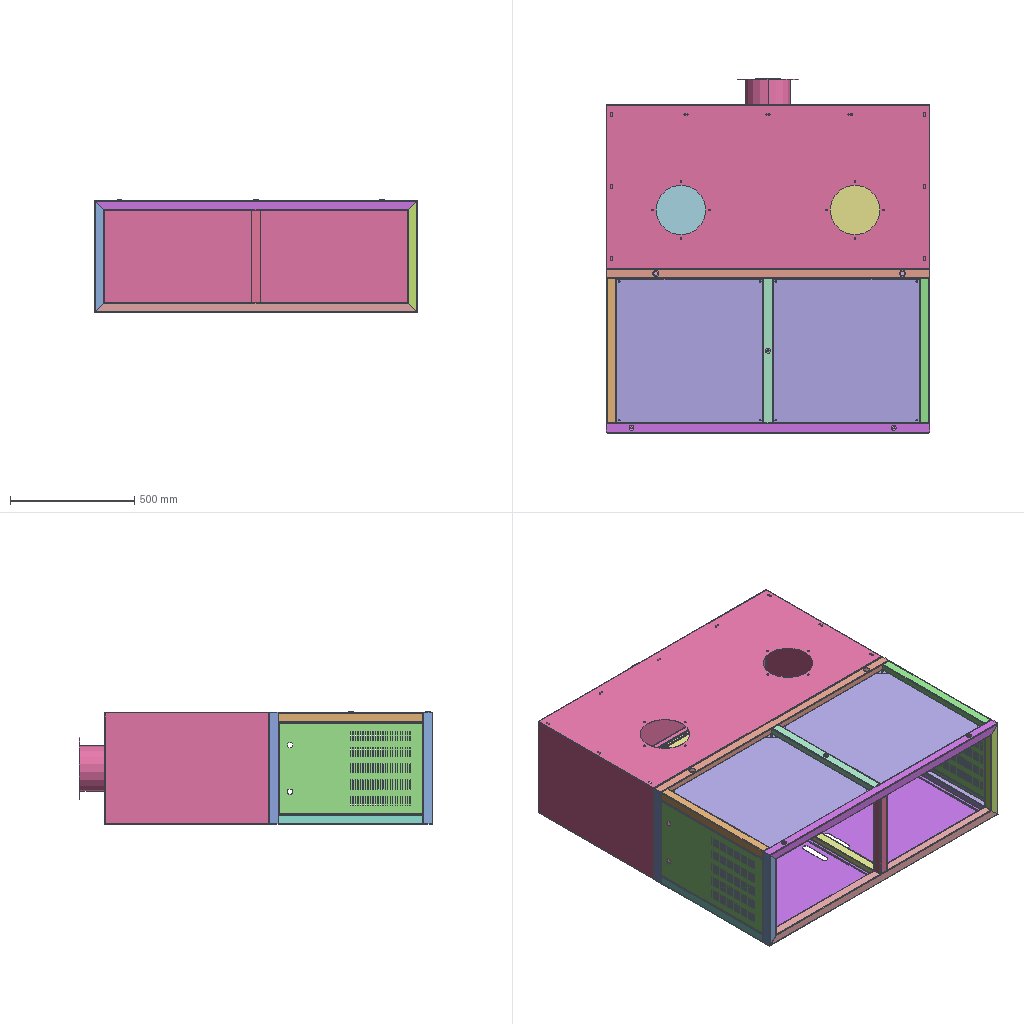Assembly | SolidWorks | 9 different items | 19 placed | box 1300 x 1423 x 453 mm
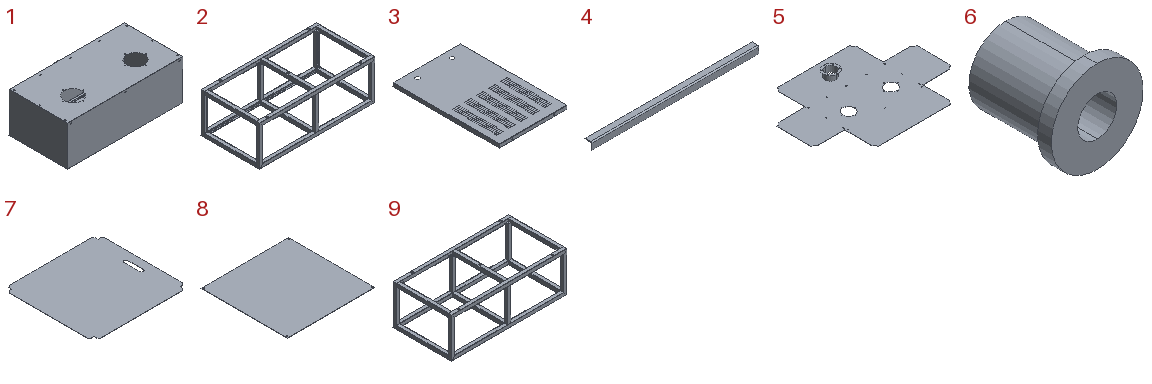Parts list (item | name | quantity | parent item | size | volume | features):
1 | (subassembly) | x1 | - | 1300 x 763 x 450 mm | 5569322 mm3 | -
2 | (subassembly) | x1 | - | 1300 x 660 x 453 mm | 3352763 mm3 | -
3 | - | x2 | - | 367 x 577 x 20 mm | 391645 mm3 | features Cut 3, EdgeFlange 2, LPattern 2, FlatPattern 1, ICE 1, SMBaseFlange 1, SheetMetal 1
4 | - | x4 | in 2 | 360 x 15 x 15 mm | 15045 mm3 | features EdgeFlange 1, FlatPattern 1, SMBaseFlange 1, SheetMetal 1
5 | - | x1 | in 1 | 2323 x 1683 x 104.5 mm | 4309239 mm3 | features ICE 8, EdgeFlange 4, CirPattern 1, FlatPattern 1, SMBaseFlange 1, SheetMetal 1
6 | - | x3 | in 2 | 20 x 20 x 20 mm | 3226 mm3 | features Extrusion 1, HoleWzd 1, ICE 1
7 | - | x4 | in 1 | 668.448 x 638.448 x 1.5 mm | 627538 mm3 | features EdgeFlange 2, FlatPattern 1, ICE 1, SMBaseFlange 1, SheetMetal 1
8 | - | x2 | - | 587 x 577 x 2 mm | 677090 mm3 | features FlatPattern 1, HoleWzd 1, SMBaseFlange 1, SheetMetal 1
9 | - | x1 | in 2 | 1300 x 660 x 450 mm | 3264516 mm3 | features WeldCornerFeat 9, Gusset 8, ICE 3, WeldMemberFeat 3, 3DProfileFeature 1, HoleWzd 1, WeldmentFeature 1
Mates (type | each side: item.copy, entity, surface, feature):
In the top assembly
Width | 8.1 face plane Base-Flange1 | 8.1 face plane Base-Flange1 | 9.1 face plane Structural Member3 | 9.1 face plane Structural Member3
Width | 8.1 face plane Base-Flange1 | 8.1 face plane Base-Flange1 | 9.1 face plane Structural Member1 | 9.1 face plane Structural Member2
Coincident | 9.1 face plane Gusset3 | 8.1 face plane Base-Flange1
Width | 8.2 face plane Base-Flange1 | 8.2 face plane Base-Flange1 | 9.1 face plane Structural Member3 | 9.1 face plane Structural Member3
Width | 8.2 face plane Base-Flange1 | 8.2 face plane Base-Flange1 | 9.1 face plane Structural Member1 | 9.1 face plane Structural Member2
Coincident | 9.1 face plane Gusset6 | 8.2 face plane Base-Flange1
Width | 3.1 face plane Edge-Flange1 | 3.1 face plane Edge-Flange1 | 9.1 face plane Structural Member3 | 9.1 face plane Structural Member3
Width | 3.1 face plane Edge-Flange1 | 3.1 face plane Edge-Flange1 | 9.1 face plane Structural Member1 | 9.1 face plane Structural Member2
Coincident | 9.1 face plane Structural Member2 | 3.1 face plane Base-Flange1
Width | 3.2 face plane Edge-Flange1 | 3.2 face plane Edge-Flange1 | 9.1 face plane Structural Member3 | 9.1 face plane Structural Member3
Coincident | 9.1 face plane Structural Member2 | 3.2 face plane Base-Flange1
Width | 3.2 face plane Edge-Flange1 | 3.2 face plane Edge-Flange1 | 9.1 face plane Structural Member1 | 9.1 face plane Structural Member2
Coincident | 9.1 face plane Structural Member2 | 5.1 face plane Edge-Flange1 | 2 times
Coincident | 9.1 face plane Structural Member2 | 5.1 face plane Edge-Flange2
Width | 7.1 face plane Edge-Flange1 | 7.1 face plane Edge-Flange1 | 9.1 face plane Structural Member1 | 9.1 face plane Structural Member2
Width | 7.1 face plane Edge-Flange1 | 7.1 face plane Edge-Flange1 | 9.1 face plane Structural Member3 | 9.1 face plane Structural Member3
Coincident | 9.1 face plane Structural Member3 | 7.1 face plane Base-Flange1
Width | 7.2 face plane Edge-Flange1 | 7.2 face plane Edge-Flange1 | 9.1 face plane Structural Member3 | 9.1 face plane Structural Member3
Width | 7.2 face plane Edge-Flange1 | 7.2 face plane Edge-Flange1 | 9.1 face plane Structural Member1 | 9.1 face plane Structural Member2
Coincident | 9.1 face plane Structural Member2 | 7.2 face plane Base-Flange1
In subassembly 2
Concentric | 9.2 face cylinder Cut-Extrude1 | 6.1 face cylinder Boss-Extrude1
Coincident | 9.2 face plane Structural Member1 | 6.1 face plane Boss-Extrude3
Concentric | 9.2 face cylinder Cut-Extrude1 | 6.2 face cylinder Boss-Extrude1
Coincident | 9.2 face plane Structural Member1 | 6.2 face plane Boss-Extrude3
Concentric | 9.2 face cylinder Cut-Extrude1 | 6.3 face cylinder Boss-Extrude1
Coincident | 9.2 face plane Structural Member3 | 6.3 face plane Boss-Extrude3
Coincident | 9.2 face plane Structural Member2 | 4.1 face plane Edge-Flange1
Width | 4.1 face plane Edge-Flange1 | 4.1 face plane Edge-Flange1 | 9.2 face plane Structural Member3 | 9.2 face plane Structural Member3
DistanceDim | 9.2 face plane Structural Member2 | 4.1 face plane Base-Flange1
Width | 4.2 face plane Edge-Flange1 | 4.2 face plane Edge-Flange1 | 9.2 face plane Structural Member3 | 9.2 face plane Structural Member3
Coincident | 9.2 face plane Structural Member2 | 4.2 face plane Edge-Flange1
DistanceDim | 4.2 face plane Base-Flange1 | 9.2 face plane Structural Member2
Width | 4.3 face plane Base-Flange1 | 4.3 face plane Base-Flange1 | 9.2 face plane Structural Member3 | 9.2 face plane Structural Member3
Coincident | 9.2 face plane Structural Member2 | 4.3 face plane Edge-Flange1
DistanceDim | 4.3 face plane Base-Flange1 | 9.2 face plane Structural Member2
Width | 4.4 face plane Base-Flange1 | 4.4 face plane Base-Flange1 | 9.2 face plane Structural Member3 | 9.2 face plane Structural Member3
Coincident | 9.2 face plane Structural Member2 | 4.4 face plane Edge-Flange1
DistanceDim | 4.4 face plane Base-Flange1 | 9.2 face plane Structural Member2
In subassembly 1
Width | 7.3 face plane Edge-Flange1 | 7.3 face plane Edge-Flange1 | 5.2 face plane Edge-Flange3 | 5.2 face plane Edge-Flange3
DistanceDim | 7.3 face plane Edge-Flange1 | 5.2 face plane Edge-Flange3
Coincident | 5.2 face plane Edge-Flange2 | 7.3 face plane Base-Flange1
Width | 7.1 face plane Edge-Flange1 | 7.1 face plane Edge-Flange1 | 5.2 face plane Edge-Flange3 | 5.2 face plane Edge-Flange3
Coincident | 5.2 face plane Edge-Flange2 | 7.1 face plane Base-Flange1
DistanceDim | 5.2 face plane Edge-Flange3 | 7.1 face plane Edge-Flange1